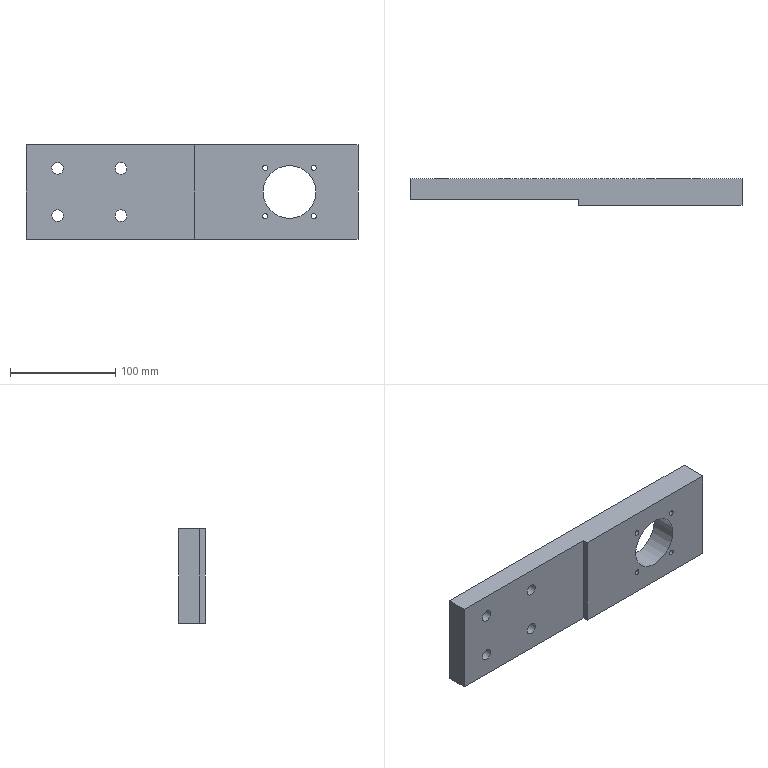Part | STEP file | SN10_003_002_PLACA | 1 solid | 17 faces | box 315 x 25 x 90 mm | volume 578161 mm3 | cylinder 9 | plane 8 | commonest cylinder face diameters 4.917 x4 11 x4 50 x1
STEP:
#1=CARTESIAN_POINT('',(0.,0.,0.));
#2=DIRECTION('',(0.,0.,1.));
#3=DIRECTION('',(1.,0.,0.));
#4=AXIS2_PLACEMENT_3D('',#1,#2,#3);
#5=CARTESIAN_POINT('',(5784.827,200.,25.137));
#6=VERTEX_POINT('',#5);
#7=CARTESIAN_POINT('',(5780.,200.,22.5));
#8=DIRECTION('',(0.,-1.,0.));
#9=DIRECTION('',(1.,0.,0.));
#10=AXIS2_PLACEMENT_3D('',#7,#8,#9);
#11=CIRCLE('',#10,5.5);
#12=CARTESIAN_POINT('',(5780.,199.9,22.5));
#13=DIRECTION('',(0.,-1.,0.));
#14=DIRECTION('',(0.8776,0.,0.4794));
#15=AXIS2_PLACEMENT_3D('',#12,#13,#14);
#16=CYLINDRICAL_SURFACE('',#15,5.5);
#17=CARTESIAN_POINT('',(-0.5,-0.1));
#18=DIRECTION('',(1.,0.));
#19=VECTOR('',#18,1.);
#20=LINE('',#17,#19);
#21=(GEOMETRIC_REPRESENTATION_CONTEXT(2)PARAMETRIC_REPRESENTATION_CONTEXT()REPRESENTATION_CONTEXT('',''));
#22=DEFINITIONAL_REPRESENTATION('',(#20),#21);
#23=PCURVE('',#16,#22);
#24=CARTESIAN_POINT('',(6065.,200.,45.));
#25=DIRECTION('',(0.,-1.,0.));
#26=DIRECTION('',(0.,0.,-1.));
#27=AXIS2_PLACEMENT_3D('',#24,#25,#26);
#28=PLANE('',#27);
#29=CARTESIAN_POINT('',(22.5,-285.));
#30=DIRECTION('',(0.,1.));
#31=AXIS2_PLACEMENT_2D('',#29,#30);
#32=CIRCLE('',#31,5.5);
#33=(GEOMETRIC_REPRESENTATION_CONTEXT(2)PARAMETRIC_REPRESENTATION_CONTEXT()REPRESENTATION_CONTEXT('',''));
#34=DEFINITIONAL_REPRESENTATION('',(#32),#33);
#35=PCURVE('',#28,#34);
#36=SURFACE_CURVE('',#11,(#23,#35),.PCURVE_S1.);
#37=EDGE_CURVE('',#6,#6,#36,.T.);
#38=ORIENTED_EDGE('',*,*,#37,.T.);
#39=CARTESIAN_POINT('',(5784.827,180.,25.137));
#40=VERTEX_POINT('',#39);
#41=CARTESIAN_POINT('',(5784.827,200.,25.137));
#42=CARTESIAN_POINT('',(5784.827,180.,25.137));
#43=B_SPLINE_CURVE_WITH_KNOTS('',1,(#41,#42),.UNSPECIFIED.,.F.,.F.,(2,2),(-0.1,19.9),.PIECEWISE_BEZIER_KNOTS.);
#44=CARTESIAN_POINT('',(6.283,0.));
#45=DIRECTION('',(0.,1.));
#46=VECTOR('',#45,1.);
#47=LINE('',#44,#46);
#48=(GEOMETRIC_REPRESENTATION_CONTEXT(2)PARAMETRIC_REPRESENTATION_CONTEXT()REPRESENTATION_CONTEXT('',''));
#49=DEFINITIONAL_REPRESENTATION('',(#47),#48);
#50=PCURVE('',#16,#49);
#51=CARTESIAN_POINT('',(0.,0.));
#52=DIRECTION('',(0.,1.));
#53=VECTOR('',#52,1.);
#54=LINE('',#51,#53);
#55=(GEOMETRIC_REPRESENTATION_CONTEXT(2)PARAMETRIC_REPRESENTATION_CONTEXT()REPRESENTATION_CONTEXT('',''));
#56=DEFINITIONAL_REPRESENTATION('',(#54),#55);
#57=PCURVE('',#16,#56);
#58=SEAM_CURVE('',#43,(#50,#57),.PCURVE_S1.);
#59=EDGE_CURVE('',#6,#40,#58,.T.);
#60=ORIENTED_EDGE('',*,*,#59,.T.);
#61=CARTESIAN_POINT('',(5780.,180.,22.5));
#62=DIRECTION('',(0.,-1.,0.));
#63=DIRECTION('',(1.,0.,0.));
#64=AXIS2_PLACEMENT_3D('',#61,#62,#63);
#65=CIRCLE('',#64,5.5);
#66=CARTESIAN_POINT('',(-0.5,19.9));
#67=DIRECTION('',(1.,0.));
#68=VECTOR('',#67,1.);
#69=LINE('',#66,#68);
#70=(GEOMETRIC_REPRESENTATION_CONTEXT(2)PARAMETRIC_REPRESENTATION_CONTEXT()REPRESENTATION_CONTEXT('',''));
#71=DEFINITIONAL_REPRESENTATION('',(#69),#70);
#72=PCURVE('',#16,#71);
#73=CARTESIAN_POINT('',(5750.,180.,45.));
#74=DIRECTION('',(0.,1.,0.));
#75=DIRECTION('',(0.,0.,1.));
#76=AXIS2_PLACEMENT_3D('',#73,#74,#75);
#77=PLANE('',#76);
#78=CARTESIAN_POINT('',(-22.5,35.5));
#79=CARTESIAN_POINT('',(-12.974,35.5));
#80=CARTESIAN_POINT('',(-17.737,27.25));
#81=CARTESIAN_POINT('',(-22.5,19.));
#82=CARTESIAN_POINT('',(-27.263,27.25));
#83=CARTESIAN_POINT('',(-32.026,35.5));
#84=CARTESIAN_POINT('',(-22.5,35.5));
#85=(BOUNDED_CURVE()B_SPLINE_CURVE(2,(#78,#79,#80,#81,#82,#83,#84),.UNSPECIFIED.,.T.,.F.)B_SPLINE_CURVE_WITH_KNOTS((1,2,2,2,2,1),(-2.094,0.,2.094,4.189,6.283,8.378),.UNSPECIFIED.)CURVE()GEOMETRIC_REPRESENTATION_ITEM()RATIONAL_B_SPLINE_CURVE((1.,0.5,1.,0.5,1.,0.5,1.))REPRESENTATION_ITEM(''));
#86=(GEOMETRIC_REPRESENTATION_CONTEXT(2)PARAMETRIC_REPRESENTATION_CONTEXT()REPRESENTATION_CONTEXT('',''));
#87=DEFINITIONAL_REPRESENTATION('',(#85),#86);
#88=PCURVE('',#77,#87);
#89=SURFACE_CURVE('',#65,(#72,#88),.PCURVE_S1.);
#90=EDGE_CURVE('',#40,#40,#89,.T.);
#91=ORIENTED_EDGE('',*,*,#90,.F.);
#92=ORIENTED_EDGE('',*,*,#59,.F.);
#93=EDGE_LOOP('',(#38,#60,#91,#92));
#94=FACE_BOUND('',#93,.F.);
#95=ADVANCED_FACE('',(#94),#16,.F.);
#96=CARTESIAN_POINT('',(6065.,175.,-45.));
#97=VERTEX_POINT('',#96);
#98=CARTESIAN_POINT('',(6065.,200.,-45.));
#99=VERTEX_POINT('',#98);
#100=CARTESIAN_POINT('',(6065.,175.,-45.));
#101=DIRECTION('',(0.,1.,0.));
#102=VECTOR('',#101,1.);
#103=LINE('',#100,#102);
#104=CARTESIAN_POINT('',(6065.,175.,45.));
#105=DIRECTION('',(-1.,0.,0.));
#106=DIRECTION('',(0.,0.,1.));
#107=AXIS2_PLACEMENT_3D('',#104,#105,#106);
#108=PLANE('',#107);
#109=CARTESIAN_POINT('',(-90.,0.));
#110=DIRECTION('',(0.,1.));
#111=VECTOR('',#110,1.);
#112=LINE('',#109,#111);
#113=(GEOMETRIC_REPRESENTATION_CONTEXT(2)PARAMETRIC_REPRESENTATION_CONTEXT()REPRESENTATION_CONTEXT('',''));
#114=DEFINITIONAL_REPRESENTATION('',(#112),#113);
#115=PCURVE('',#108,#114);
#116=CARTESIAN_POINT('',(0.,0.,-45.));
#117=DIRECTION('',(0.,0.,1.));
#118=DIRECTION('',(1.,0.,0.));
#119=AXIS2_PLACEMENT_3D('',#116,#117,#118);
#120=PLANE('',#119);
#121=CARTESIAN_POINT('',(6065.,175.));
#122=DIRECTION('',(0.,1.));
#123=VECTOR('',#122,1.);
#124=LINE('',#121,#123);
#125=(GEOMETRIC_REPRESENTATION_CONTEXT(2)PARAMETRIC_REPRESENTATION_CONTEXT()REPRESENTATION_CONTEXT('',''));
#126=DEFINITIONAL_REPRESENTATION('',(#124),#125);
#127=PCURVE('',#120,#126);
#128=SURFACE_CURVE('',#103,(#115,#127),.PCURVE_S1.);
#129=EDGE_CURVE('',#97,#99,#128,.T.);
#130=ORIENTED_EDGE('',*,*,#129,.T.);
#131=CARTESIAN_POINT('',(6065.,200.,45.));
#132=VERTEX_POINT('',#131);
#133=CARTESIAN_POINT('',(6065.,200.,45.));
#134=DIRECTION('',(0.,0.,-1.));
#135=VECTOR('',#134,1.);
#136=LINE('',#133,#135);
#137=CARTESIAN_POINT('',(0.,25.));
#138=DIRECTION('',(-1.,0.));
#139=VECTOR('',#138,1.);
#140=LINE('',#137,#139);
#141=(GEOMETRIC_REPRESENTATION_CONTEXT(2)PARAMETRIC_REPRESENTATION_CONTEXT()REPRESENTATION_CONTEXT('',''));
#142=DEFINITIONAL_REPRESENTATION('',(#140),#141);
#143=PCURVE('',#108,#142);
#144=CARTESIAN_POINT('',(0.,0.));
#145=DIRECTION('',(1.,0.));
#146=VECTOR('',#145,1.);
#147=LINE('',#144,#146);
#148=(GEOMETRIC_REPRESENTATION_CONTEXT(2)PARAMETRIC_REPRESENTATION_CONTEXT()REPRESENTATION_CONTEXT('',''));
#149=DEFINITIONAL_REPRESENTATION('',(#147),#148);
#150=PCURVE('',#28,#149);
#151=SURFACE_CURVE('',#136,(#143,#150),.PCURVE_S1.);
#152=EDGE_CURVE('',#132,#99,#151,.T.);
#153=ORIENTED_EDGE('',*,*,#152,.F.);
#154=CARTESIAN_POINT('',(6065.,175.,45.));
#155=VERTEX_POINT('',#154);
#156=CARTESIAN_POINT('',(6065.,175.,45.));
#157=DIRECTION('',(0.,1.,0.));
#158=VECTOR('',#157,1.);
#159=LINE('',#156,#158);
#160=CARTESIAN_POINT('',(0.,0.));
#161=DIRECTION('',(0.,1.));
#162=VECTOR('',#161,1.);
#163=LINE('',#160,#162);
#164=(GEOMETRIC_REPRESENTATION_CONTEXT(2)PARAMETRIC_REPRESENTATION_CONTEXT()REPRESENTATION_CONTEXT('',''));
#165=DEFINITIONAL_REPRESENTATION('',(#163),#164);
#166=PCURVE('',#108,#165);
#167=CARTESIAN_POINT('',(0.,0.,45.));
#168=DIRECTION('',(0.,0.,1.));
#169=DIRECTION('',(1.,0.,0.));
#170=AXIS2_PLACEMENT_3D('',#167,#168,#169);
#171=PLANE('',#170);
#172=CARTESIAN_POINT('',(6065.,175.));
#173=DIRECTION('',(0.,1.));
#174=VECTOR('',#173,1.);
#175=LINE('',#172,#174);
#176=(GEOMETRIC_REPRESENTATION_CONTEXT(2)PARAMETRIC_REPRESENTATION_CONTEXT()REPRESENTATION_CONTEXT('',''));
#177=DEFINITIONAL_REPRESENTATION('',(#175),#176);
#178=PCURVE('',#171,#177);
#179=SURFACE_CURVE('',#159,(#166,#178),.PCURVE_S1.);
#180=EDGE_CURVE('',#155,#132,#179,.T.);
#181=ORIENTED_EDGE('',*,*,#180,.F.);
#182=CARTESIAN_POINT('',(6065.,175.,45.));
#183=DIRECTION('',(0.,0.,-1.));
#184=VECTOR('',#183,1.);
#185=LINE('',#182,#184);
#186=CARTESIAN_POINT('',(0.,0.));
#187=DIRECTION('',(-1.,0.));
#188=VECTOR('',#187,1.);
#189=LINE('',#186,#188);
#190=(GEOMETRIC_REPRESENTATION_CONTEXT(2)PARAMETRIC_REPRESENTATION_CONTEXT()REPRESENTATION_CONTEXT('',''));
#191=DEFINITIONAL_REPRESENTATION('',(#189),#190);
#192=PCURVE('',#108,#191);
#193=CARTESIAN_POINT('',(5910.,175.,45.));
#194=DIRECTION('',(0.,1.,0.));
#195=DIRECTION('',(0.,0.,1.));
#196=AXIS2_PLACEMENT_3D('',#193,#194,#195);
#197=PLANE('',#196);
#198=CARTESIAN_POINT('',(0.,155.));
#199=DIRECTION('',(-1.,0.));
#200=VECTOR('',#199,1.);
#201=LINE('',#198,#200);
#202=(GEOMETRIC_REPRESENTATION_CONTEXT(2)PARAMETRIC_REPRESENTATION_CONTEXT()REPRESENTATION_CONTEXT('',''));
#203=DEFINITIONAL_REPRESENTATION('',(#201),#202);
#204=PCURVE('',#197,#203);
#205=SURFACE_CURVE('',#185,(#192,#204),.PCURVE_S1.);
#206=EDGE_CURVE('',#155,#97,#205,.T.);
#207=ORIENTED_EDGE('',*,*,#206,.T.);
#208=EDGE_LOOP('',(#130,#153,#181,#207));
#209=FACE_BOUND('',#208,.T.);
#210=ADVANCED_FACE('',(#209),#108,.F.);
#211=CARTESIAN_POINT('',(5750.,200.,-45.));
#212=VERTEX_POINT('',#211);
#213=CARTESIAN_POINT('',(5750.,180.,-45.));
#214=VERTEX_POINT('',#213);
#215=CARTESIAN_POINT('',(5750.,200.,-45.));
#216=DIRECTION('',(0.,-1.,0.));
#217=VECTOR('',#216,1.);
#218=LINE('',#215,#217);
#219=CARTESIAN_POINT('',(5750.,200.));
#220=DIRECTION('',(0.,-1.));
#221=VECTOR('',#220,1.);
#222=LINE('',#219,#221);
#223=(GEOMETRIC_REPRESENTATION_CONTEXT(2)PARAMETRIC_REPRESENTATION_CONTEXT()REPRESENTATION_CONTEXT('',''));
#224=DEFINITIONAL_REPRESENTATION('',(#222),#223);
#225=PCURVE('',#120,#224);
#226=CARTESIAN_POINT('',(5750.,200.,45.));
#227=DIRECTION('',(1.,0.,0.));
#228=DIRECTION('',(0.,0.,-1.));
#229=AXIS2_PLACEMENT_3D('',#226,#227,#228);
#230=PLANE('',#229);
#231=CARTESIAN_POINT('',(90.,0.));
#232=DIRECTION('',(0.,-1.));
#233=VECTOR('',#232,1.);
#234=LINE('',#231,#233);
#235=(GEOMETRIC_REPRESENTATION_CONTEXT(2)PARAMETRIC_REPRESENTATION_CONTEXT()REPRESENTATION_CONTEXT('',''));
#236=DEFINITIONAL_REPRESENTATION('',(#234),#235);
#237=PCURVE('',#230,#236);
#238=SURFACE_CURVE('',#218,(#225,#237),.PCURVE_S1.);
#239=EDGE_CURVE('',#212,#214,#238,.T.);
#240=ORIENTED_EDGE('',*,*,#239,.F.);
#241=CARTESIAN_POINT('',(6065.,200.,-45.));
#242=DIRECTION('',(-1.,0.,0.));
#243=VECTOR('',#242,1.);
#244=LINE('',#241,#243);
#245=CARTESIAN_POINT('',(6065.,200.));
#246=DIRECTION('',(-1.,0.));
#247=VECTOR('',#246,1.);
#248=LINE('',#245,#247);
#249=(GEOMETRIC_REPRESENTATION_CONTEXT(2)PARAMETRIC_REPRESENTATION_CONTEXT()REPRESENTATION_CONTEXT('',''));
#250=DEFINITIONAL_REPRESENTATION('',(#248),#249);
#251=PCURVE('',#120,#250);
#252=CARTESIAN_POINT('',(90.,0.));
#253=DIRECTION('',(0.,-1.));
#254=VECTOR('',#253,1.);
#255=LINE('',#252,#254);
#256=(GEOMETRIC_REPRESENTATION_CONTEXT(2)PARAMETRIC_REPRESENTATION_CONTEXT()REPRESENTATION_CONTEXT('',''));
#257=DEFINITIONAL_REPRESENTATION('',(#255),#256);
#258=PCURVE('',#28,#257);
#259=SURFACE_CURVE('',#244,(#251,#258),.PCURVE_S1.);
#260=EDGE_CURVE('',#99,#212,#259,.T.);
#261=ORIENTED_EDGE('',*,*,#260,.F.);
#262=ORIENTED_EDGE('',*,*,#129,.F.);
#263=CARTESIAN_POINT('',(5910.,175.,-45.));
#264=VERTEX_POINT('',#263);
#265=CARTESIAN_POINT('',(5910.,175.,-45.));
#266=DIRECTION('',(1.,0.,0.));
#267=VECTOR('',#266,1.);
#268=LINE('',#265,#267);
#269=CARTESIAN_POINT('',(5910.,175.));
#270=DIRECTION('',(1.,0.));
#271=VECTOR('',#270,1.);
#272=LINE('',#269,#271);
#273=(GEOMETRIC_REPRESENTATION_CONTEXT(2)PARAMETRIC_REPRESENTATION_CONTEXT()REPRESENTATION_CONTEXT('',''));
#274=DEFINITIONAL_REPRESENTATION('',(#272),#273);
#275=PCURVE('',#120,#274);
#276=CARTESIAN_POINT('',(-90.,0.));
#277=DIRECTION('',(0.,1.));
#278=VECTOR('',#277,1.);
#279=LINE('',#276,#278);
#280=(GEOMETRIC_REPRESENTATION_CONTEXT(2)PARAMETRIC_REPRESENTATION_CONTEXT()REPRESENTATION_CONTEXT('',''));
#281=DEFINITIONAL_REPRESENTATION('',(#279),#280);
#282=PCURVE('',#197,#281);
#283=SURFACE_CURVE('',#268,(#275,#282),.PCURVE_S1.);
#284=EDGE_CURVE('',#264,#97,#283,.T.);
#285=ORIENTED_EDGE('',*,*,#284,.F.);
#286=CARTESIAN_POINT('',(5910.,180.,-45.));
#287=VERTEX_POINT('',#286);
#288=CARTESIAN_POINT('',(5910.,180.,-45.));
#289=DIRECTION('',(0.,-1.,0.));
#290=VECTOR('',#289,1.);
#291=LINE('',#288,#290);
#292=CARTESIAN_POINT('',(5910.,180.));
#293=DIRECTION('',(0.,-1.));
#294=VECTOR('',#293,1.);
#295=LINE('',#292,#294);
#296=(GEOMETRIC_REPRESENTATION_CONTEXT(2)PARAMETRIC_REPRESENTATION_CONTEXT()REPRESENTATION_CONTEXT('',''));
#297=DEFINITIONAL_REPRESENTATION('',(#295),#296);
#298=PCURVE('',#120,#297);
#299=CARTESIAN_POINT('',(5910.,180.,45.));
#300=DIRECTION('',(1.,0.,0.));
#301=DIRECTION('',(0.,0.,-1.));
#302=AXIS2_PLACEMENT_3D('',#299,#300,#301);
#303=PLANE('',#302);
#304=CARTESIAN_POINT('',(90.,0.));
#305=DIRECTION('',(0.,-1.));
#306=VECTOR('',#305,1.);
#307=LINE('',#304,#306);
#308=(GEOMETRIC_REPRESENTATION_CONTEXT(2)PARAMETRIC_REPRESENTATION_CONTEXT()REPRESENTATION_CONTEXT('',''));
#309=DEFINITIONAL_REPRESENTATION('',(#307),#308);
#310=PCURVE('',#303,#309);
#311=SURFACE_CURVE('',#291,(#298,#310),.PCURVE_S1.);
#312=EDGE_CURVE('',#287,#264,#311,.T.);
#313=ORIENTED_EDGE('',*,*,#312,.F.);
#314=CARTESIAN_POINT('',(5750.,180.,-45.));
#315=DIRECTION('',(1.,0.,0.));
#316=VECTOR('',#315,1.);
#317=LINE('',#314,#316);
#318=CARTESIAN_POINT('',(5750.,180.));
#319=DIRECTION('',(1.,0.));
#320=VECTOR('',#319,1.);
#321=LINE('',#318,#320);
#322=(GEOMETRIC_REPRESENTATION_CONTEXT(2)PARAMETRIC_REPRESENTATION_CONTEXT()REPRESENTATION_CONTEXT('',''));
#323=DEFINITIONAL_REPRESENTATION('',(#321),#322);
#324=PCURVE('',#120,#323);
#325=CARTESIAN_POINT('',(-90.,0.));
#326=DIRECTION('',(0.,1.));
#327=VECTOR('',#326,1.);
#328=LINE('',#325,#327);
#329=(GEOMETRIC_REPRESENTATION_CONTEXT(2)PARAMETRIC_REPRESENTATION_CONTEXT()REPRESENTATION_CONTEXT('',''));
#330=DEFINITIONAL_REPRESENTATION('',(#328),#329);
#331=PCURVE('',#77,#330);
#332=SURFACE_CURVE('',#317,(#324,#331),.PCURVE_S1.);
#333=EDGE_CURVE('',#214,#287,#332,.T.);
#334=ORIENTED_EDGE('',*,*,#333,.F.);
#335=EDGE_LOOP('',(#240,#261,#262,#285,#313,#334));
#336=FACE_BOUND('',#335,.T.);
#337=ADVANCED_FACE('',(#336),#120,.F.);
#338=CARTESIAN_POINT('',(6020.823,200.,21.802));
#339=VERTEX_POINT('',#338);
#340=CARTESIAN_POINT('',(6022.981,200.,22.981));
#341=DIRECTION('',(0.,-1.,0.));
#342=DIRECTION('',(1.,0.,0.));
#343=AXIS2_PLACEMENT_3D('',#340,#341,#342);
#344=CIRCLE('',#343,2.458);
#345=CARTESIAN_POINT('',(6022.981,199.9,22.981));
#346=DIRECTION('',(0.,-1.,0.));
#347=DIRECTION('',(0.8776,0.,0.4794));
#348=AXIS2_PLACEMENT_3D('',#345,#346,#347);
#349=CYLINDRICAL_SURFACE('',#348,2.458);
#350=CARTESIAN_POINT('',(-0.5,-0.1));
#351=DIRECTION('',(1.,0.));
#352=VECTOR('',#351,1.);
#353=LINE('',#350,#352);
#354=(GEOMETRIC_REPRESENTATION_CONTEXT(2)PARAMETRIC_REPRESENTATION_CONTEXT()REPRESENTATION_CONTEXT('',''));
#355=DEFINITIONAL_REPRESENTATION('',(#353),#354);
#356=PCURVE('',#349,#355);
#357=CARTESIAN_POINT('',(22.019,-42.019));
#358=DIRECTION('',(0.,1.));
#359=AXIS2_PLACEMENT_2D('',#357,#358);
#360=CIRCLE('',#359,2.458);
#361=(GEOMETRIC_REPRESENTATION_CONTEXT(2)PARAMETRIC_REPRESENTATION_CONTEXT()REPRESENTATION_CONTEXT('',''));
#362=DEFINITIONAL_REPRESENTATION('',(#360),#361);
#363=PCURVE('',#28,#362);
#364=SURFACE_CURVE('',#344,(#356,#363),.PCURVE_S1.);
#365=EDGE_CURVE('',#339,#339,#364,.T.);
#366=ORIENTED_EDGE('',*,*,#365,.T.);
#367=CARTESIAN_POINT('',(6020.823,175.,21.802));
#368=VERTEX_POINT('',#367);
#369=CARTESIAN_POINT('',(6020.823,200.,21.802));
#370=CARTESIAN_POINT('',(6020.823,175.,21.802));
#371=B_SPLINE_CURVE_WITH_KNOTS('',1,(#369,#370),.UNSPECIFIED.,.F.,.F.,(2,2),(-0.1,24.9),.PIECEWISE_BEZIER_KNOTS.);
#372=CARTESIAN_POINT('',(9.425,0.));
#373=DIRECTION('',(0.,1.));
#374=VECTOR('',#373,1.);
#375=LINE('',#372,#374);
#376=(GEOMETRIC_REPRESENTATION_CONTEXT(2)PARAMETRIC_REPRESENTATION_CONTEXT()REPRESENTATION_CONTEXT('',''));
#377=DEFINITIONAL_REPRESENTATION('',(#375),#376);
#378=PCURVE('',#349,#377);
#379=CARTESIAN_POINT('',(3.142,0.));
#380=DIRECTION('',(0.,1.));
#381=VECTOR('',#380,1.);
#382=LINE('',#379,#381);
#383=(GEOMETRIC_REPRESENTATION_CONTEXT(2)PARAMETRIC_REPRESENTATION_CONTEXT()REPRESENTATION_CONTEXT('',''));
#384=DEFINITIONAL_REPRESENTATION('',(#382),#383);
#385=PCURVE('',#349,#384);
#386=SEAM_CURVE('',#371,(#378,#385),.PCURVE_S1.);
#387=EDGE_CURVE('',#339,#368,#386,.T.);
#388=ORIENTED_EDGE('',*,*,#387,.T.);
#389=CARTESIAN_POINT('',(6022.981,175.,22.981));
#390=DIRECTION('',(0.,-1.,0.));
#391=DIRECTION('',(1.,0.,0.));
#392=AXIS2_PLACEMENT_3D('',#389,#390,#391);
#393=CIRCLE('',#392,2.458);
#394=CARTESIAN_POINT('',(-0.5,24.9));
#395=DIRECTION('',(1.,0.));
#396=VECTOR('',#395,1.);
#397=LINE('',#394,#396);
#398=(GEOMETRIC_REPRESENTATION_CONTEXT(2)PARAMETRIC_REPRESENTATION_CONTEXT()REPRESENTATION_CONTEXT('',''));
#399=DEFINITIONAL_REPRESENTATION('',(#397),#398);
#400=PCURVE('',#349,#399);
#401=CARTESIAN_POINT('',(-22.019,115.439));
#402=CARTESIAN_POINT('',(-17.761,115.439));
#403=CARTESIAN_POINT('',(-19.89,111.752));
#404=CARTESIAN_POINT('',(-22.019,108.064));
#405=CARTESIAN_POINT('',(-24.148,111.752));
#406=CARTESIAN_POINT('',(-26.277,115.439));
#407=CARTESIAN_POINT('',(-22.019,115.439));
#408=(BOUNDED_CURVE()B_SPLINE_CURVE(2,(#401,#402,#403,#404,#405,#406,#407),.UNSPECIFIED.,.T.,.F.)B_SPLINE_CURVE_WITH_KNOTS((1,2,2,2,2,1),(-2.094,0.,2.094,4.189,6.283,8.378),.UNSPECIFIED.)CURVE()GEOMETRIC_REPRESENTATION_ITEM()RATIONAL_B_SPLINE_CURVE((1.,0.5,1.,0.5,1.,0.5,1.))REPRESENTATION_ITEM(''));
#409=(GEOMETRIC_REPRESENTATION_CONTEXT(2)PARAMETRIC_REPRESENTATION_CONTEXT()REPRESENTATION_CONTEXT('',''));
#410=DEFINITIONAL_REPRESENTATION('',(#408),#409);
#411=PCURVE('',#197,#410);
#412=SURFACE_CURVE('',#393,(#400,#411),.PCURVE_S1.);
#413=EDGE_CURVE('',#368,#368,#412,.T.);
#414=ORIENTED_EDGE('',*,*,#413,.F.);
#415=ORIENTED_EDGE('',*,*,#387,.F.);
#416=EDGE_LOOP('',(#366,#388,#414,#415));
#417=FACE_BOUND('',#416,.F.);
#418=ADVANCED_FACE('',(#417),#349,.F.);
#419=CARTESIAN_POINT('',(5975.,200.,0.));
#420=VERTEX_POINT('',#419);
#421=CARTESIAN_POINT('',(6000.,200.,0.));
#422=DIRECTION('',(0.,-1.,0.));
#423=DIRECTION('',(1.,0.,0.));
#424=AXIS2_PLACEMENT_3D('',#421,#422,#423);
#425=CIRCLE('',#424,25.);
#426=CARTESIAN_POINT('',(6000.,188.16,0.));
#427=DIRECTION('',(0.,-1.,0.));
#428=DIRECTION('',(1.,0.,0.));
#429=AXIS2_PLACEMENT_3D('',#426,#427,#428);
#430=CYLINDRICAL_SURFACE('',#429,25.);
#431=CARTESIAN_POINT('',(0.,-11.84));
#432=DIRECTION('',(1.,0.));
#433=VECTOR('',#432,1.);
#434=LINE('',#431,#433);
#435=(GEOMETRIC_REPRESENTATION_CONTEXT(2)PARAMETRIC_REPRESENTATION_CONTEXT()REPRESENTATION_CONTEXT('',''));
#436=DEFINITIONAL_REPRESENTATION('',(#434),#435);
#437=PCURVE('',#430,#436);
#438=CARTESIAN_POINT('',(45.,-65.));
#439=DIRECTION('',(0.,1.));
#440=AXIS2_PLACEMENT_2D('',#438,#439);
#441=CIRCLE('',#440,25.);
#442=(GEOMETRIC_REPRESENTATION_CONTEXT(2)PARAMETRIC_REPRESENTATION_CONTEXT()REPRESENTATION_CONTEXT('',''));
#443=DEFINITIONAL_REPRESENTATION('',(#441),#442);
#444=PCURVE('',#28,#443);
#445=SURFACE_CURVE('',#425,(#437,#444),.PCURVE_S1.);
#446=EDGE_CURVE('',#420,#420,#445,.T.);
#447=ORIENTED_EDGE('',*,*,#446,.T.);
#448=CARTESIAN_POINT('',(5975.,175.,0.));
#449=VERTEX_POINT('',#448);
#450=CARTESIAN_POINT('',(5975.,200.,0.));
#451=CARTESIAN_POINT('',(5975.,175.,0.));
#452=B_SPLINE_CURVE_WITH_KNOTS('',1,(#450,#451),.UNSPECIFIED.,.F.,.F.,(2,2),(-11.84,13.16),.PIECEWISE_BEZIER_KNOTS.);
#453=CARTESIAN_POINT('',(9.425,0.));
#454=DIRECTION('',(0.,1.));
#455=VECTOR('',#454,1.);
#456=LINE('',#453,#455);
#457=(GEOMETRIC_REPRESENTATION_CONTEXT(2)PARAMETRIC_REPRESENTATION_CONTEXT()REPRESENTATION_CONTEXT('',''));
#458=DEFINITIONAL_REPRESENTATION('',(#456),#457);
#459=PCURVE('',#430,#458);
#460=CARTESIAN_POINT('',(3.142,0.));
#461=DIRECTION('',(0.,1.));
#462=VECTOR('',#461,1.);
#463=LINE('',#460,#462);
#464=(GEOMETRIC_REPRESENTATION_CONTEXT(2)PARAMETRIC_REPRESENTATION_CONTEXT()REPRESENTATION_CONTEXT('',''));
#465=DEFINITIONAL_REPRESENTATION('',(#463),#464);
#466=PCURVE('',#430,#465);
#467=SEAM_CURVE('',#452,(#459,#466),.PCURVE_S1.);
#468=EDGE_CURVE('',#420,#449,#467,.T.);
#469=ORIENTED_EDGE('',*,*,#468,.T.);
#470=CARTESIAN_POINT('',(6000.,175.,0.));
#471=DIRECTION('',(0.,-1.,0.));
#472=DIRECTION('',(1.,0.,0.));
#473=AXIS2_PLACEMENT_3D('',#470,#471,#472);
#474=CIRCLE('',#473,25.);
#475=CARTESIAN_POINT('',(0.,13.16));
#476=DIRECTION('',(1.,0.));
#477=VECTOR('',#476,1.);
#478=LINE('',#475,#477);
#479=(GEOMETRIC_REPRESENTATION_CONTEXT(2)PARAMETRIC_REPRESENTATION_CONTEXT()REPRESENTATION_CONTEXT('',''));
#480=DEFINITIONAL_REPRESENTATION('',(#478),#479);
#481=PCURVE('',#430,#480);
#482=CARTESIAN_POINT('',(-45.,115.));
#483=CARTESIAN_POINT('',(-1.699,115.));
#484=CARTESIAN_POINT('',(-23.349,77.5));
#485=CARTESIAN_POINT('',(-45.,40.));
#486=CARTESIAN_POINT('',(-66.651,77.5));
#487=CARTESIAN_POINT('',(-88.301,115.));
#488=CARTESIAN_POINT('',(-45.,115.));
#489=(BOUNDED_CURVE()B_SPLINE_CURVE(2,(#482,#483,#484,#485,#486,#487,#488),.UNSPECIFIED.,.T.,.F.)B_SPLINE_CURVE_WITH_KNOTS((1,2,2,2,2,1),(-2.094,0.,2.094,4.189,6.283,8.378),.UNSPECIFIED.)CURVE()GEOMETRIC_REPRESENTATION_ITEM()RATIONAL_B_SPLINE_CURVE((1.,0.5,1.,0.5,1.,0.5,1.))REPRESENTATION_ITEM(''));
#490=(GEOMETRIC_REPRESENTATION_CONTEXT(2)PARAMETRIC_REPRESENTATION_CONTEXT()REPRESENTATION_CONTEXT('',''));
#491=DEFINITIONAL_REPRESENTATION('',(#489),#490);
#492=PCURVE('',#197,#491);
#493=SURFACE_CURVE('',#474,(#481,#492),.PCURVE_S1.);
#494=EDGE_CURVE('',#449,#449,#493,.T.);
#495=ORIENTED_EDGE('',*,*,#494,.F.);
#496=ORIENTED_EDGE('',*,*,#468,.F.);
#497=EDGE_LOOP('',(#447,#469,#495,#496));
#498=FACE_BOUND('',#497,.F.);
#499=ADVANCED_FACE('',(#498),#430,.F.);
#500=CARTESIAN_POINT('',(6024.16,200.,-25.139));
#501=VERTEX_POINT('',#500);
#502=CARTESIAN_POINT('',(6022.981,200.,-22.981));
#503=DIRECTION('',(0.,-1.,0.));
#504=DIRECTION('',(1.,0.,0.));
#505=AXIS2_PLACEMENT_3D('',#502,#503,#504);
#506=CIRCLE('',#505,2.458);
#507=CARTESIAN_POINT('',(6022.981,199.9,-22.981));
#508=DIRECTION('',(0.,-1.,0.));
#509=DIRECTION('',(0.4794,0.,-0.8776));
#510=AXIS2_PLACEMENT_3D('',#507,#508,#509);
#511=CYLINDRICAL_SURFACE('',#510,2.458);
#512=CARTESIAN_POINT('',(1.071,-0.1));
#513=DIRECTION('',(1.,0.));
#514=VECTOR('',#513,1.);
#515=LINE('',#512,#514);
#516=(GEOMETRIC_REPRESENTATION_CONTEXT(2)PARAMETRIC_REPRESENTATION_CONTEXT()REPRESENTATION_CONTEXT('',''));
#517=DEFINITIONAL_REPRESENTATION('',(#515),#516);
#518=PCURVE('',#511,#517);
#519=CARTESIAN_POINT('',(67.981,-42.019));
#520=DIRECTION('',(0.,1.));
#521=AXIS2_PLACEMENT_2D('',#519,#520);
#522=CIRCLE('',#521,2.458);
#523=(GEOMETRIC_REPRESENTATION_CONTEXT(2)PARAMETRIC_REPRESENTATION_CONTEXT()REPRESENTATION_CONTEXT('',''));
#524=DEFINITIONAL_REPRESENTATION('',(#522),#523);
#525=PCURVE('',#28,#524);
#526=SURFACE_CURVE('',#506,(#518,#525),.PCURVE_S1.);
#527=EDGE_CURVE('',#501,#501,#526,.T.);
#528=ORIENTED_EDGE('',*,*,#527,.T.);
#529=CARTESIAN_POINT('',(6024.16,175.,-25.139));
#530=VERTEX_POINT('',#529);
#531=CARTESIAN_POINT('',(6024.16,200.,-25.139));
#532=CARTESIAN_POINT('',(6024.16,175.,-25.139));
#533=B_SPLINE_CURVE_WITH_KNOTS('',1,(#531,#532),.UNSPECIFIED.,.F.,.F.,(2,2),(-0.1,24.9),.PIECEWISE_BEZIER_KNOTS.);
#534=CARTESIAN_POINT('',(12.566,0.));
#535=DIRECTION('',(0.,1.));
#536=VECTOR('',#535,1.);
#537=LINE('',#534,#536);
#538=(GEOMETRIC_REPRESENTATION_CONTEXT(2)PARAMETRIC_REPRESENTATION_CONTEXT()REPRESENTATION_CONTEXT('',''));
#539=DEFINITIONAL_REPRESENTATION('',(#537),#538);
#540=PCURVE('',#511,#539);
#541=CARTESIAN_POINT('',(6.283,0.));
#542=DIRECTION('',(0.,1.));
#543=VECTOR('',#542,1.);
#544=LINE('',#541,#543);
#545=(GEOMETRIC_REPRESENTATION_CONTEXT(2)PARAMETRIC_REPRESENTATION_CONTEXT()REPRESENTATION_CONTEXT('',''));
#546=DEFINITIONAL_REPRESENTATION('',(#544),#545);
#547=PCURVE('',#511,#546);
#548=SEAM_CURVE('',#533,(#540,#547),.PCURVE_S1.);
#549=EDGE_CURVE('',#501,#530,#548,.T.);
#550=ORIENTED_EDGE('',*,*,#549,.T.);
#551=CARTESIAN_POINT('',(6022.981,175.,-22.981));
#552=DIRECTION('',(0.,-1.,0.));
#553=DIRECTION('',(1.,0.,0.));
#554=AXIS2_PLACEMENT_3D('',#551,#552,#553);
#555=CIRCLE('',#554,2.458);
#556=CARTESIAN_POINT('',(1.071,24.9));
#557=DIRECTION('',(1.,0.));
#558=VECTOR('',#557,1.);
#559=LINE('',#556,#558);
#560=(GEOMETRIC_REPRESENTATION_CONTEXT(2)PARAMETRIC_REPRESENTATION_CONTEXT()REPRESENTATION_CONTEXT('',''));
#561=DEFINITIONAL_REPRESENTATION('',(#559),#560);
#562=PCURVE('',#511,#561);
#563=CARTESIAN_POINT('',(-67.981,115.439));
#564=CARTESIAN_POINT('',(-63.723,115.439));
#565=CARTESIAN_POINT('',(-65.852,111.752));
#566=CARTESIAN_POINT('',(-67.981,108.064));
#567=CARTESIAN_POINT('',(-70.11,111.752));
#568=CARTESIAN_POINT('',(-72.239,115.439));
#569=CARTESIAN_POINT('',(-67.981,115.439));
#570=(BOUNDED_CURVE()B_SPLINE_CURVE(2,(#563,#564,#565,#566,#567,#568,#569),.UNSPECIFIED.,.T.,.F.)B_SPLINE_CURVE_WITH_KNOTS((1,2,2,2,2,1),(-2.094,0.,2.094,4.189,6.283,8.378),.UNSPECIFIED.)CURVE()GEOMETRIC_REPRESENTATION_ITEM()RATIONAL_B_SPLINE_CURVE((1.,0.5,1.,0.5,1.,0.5,1.))REPRESENTATION_ITEM(''));
#571=(GEOMETRIC_REPRESENTATION_CONTEXT(2)PARAMETRIC_REPRESENTATION_CONTEXT()REPRESENTATION_CONTEXT('',''));
#572=DEFINITIONAL_REPRESENTATION('',(#570),#571);
#573=PCURVE('',#197,#572);
#574=SURFACE_CURVE('',#555,(#562,#573),.PCURVE_S1.);
#575=EDGE_CURVE('',#530,#530,#574,.T.);
#576=ORIENTED_EDGE('',*,*,#575,.F.);
#577=ORIENTED_EDGE('',*,*,#549,.F.);
#578=EDGE_LOOP('',(#528,#550,#576,#577));
#579=FACE_BOUND('',#578,.F.);
#580=ADVANCED_FACE('',(#579),#511,.F.);
#581=CARTESIAN_POINT('',(5974.861,200.,-24.16));
#582=VERTEX_POINT('',#581);
#583=CARTESIAN_POINT('',(5977.019,200.,-22.981));
#584=DIRECTION('',(0.,-1.,0.));
#585=DIRECTION('',(1.,0.,0.));
#586=AXIS2_PLACEMENT_3D('',#583,#584,#585);
#587=CIRCLE('',#586,2.458);
#588=CARTESIAN_POINT('',(5977.019,199.9,-22.981));
#589=DIRECTION('',(0.,-1.,0.));
#590=DIRECTION('',(-0.8776,0.,-0.4794));
#591=AXIS2_PLACEMENT_3D('',#588,#589,#590);
#592=CYLINDRICAL_SURFACE('',#591,2.458);
#593=CARTESIAN_POINT('',(-3.642,-0.1));
#594=DIRECTION('',(1.,0.));
#595=VECTOR('',#594,1.);
#596=LINE('',#593,#595);
#597=(GEOMETRIC_REPRESENTATION_CONTEXT(2)PARAMETRIC_REPRESENTATION_CONTEXT()REPRESENTATION_CONTEXT('',''));
#598=DEFINITIONAL_REPRESENTATION('',(#596),#597);
#599=PCURVE('',#592,#598);
#600=CARTESIAN_POINT('',(67.981,-87.981));
#601=DIRECTION('',(0.,1.));
#602=AXIS2_PLACEMENT_2D('',#600,#601);
#603=CIRCLE('',#602,2.458);
#604=(GEOMETRIC_REPRESENTATION_CONTEXT(2)PARAMETRIC_REPRESENTATION_CONTEXT()REPRESENTATION_CONTEXT('',''));
#605=DEFINITIONAL_REPRESENTATION('',(#603),#604);
#606=PCURVE('',#28,#605);
#607=SURFACE_CURVE('',#587,(#599,#606),.PCURVE_S1.);
#608=EDGE_CURVE('',#582,#582,#607,.T.);
#609=ORIENTED_EDGE('',*,*,#608,.T.);
#610=CARTESIAN_POINT('',(5974.861,175.,-24.16));
#611=VERTEX_POINT('',#610);
#612=CARTESIAN_POINT('',(5974.861,200.,-24.16));
#613=CARTESIAN_POINT('',(5974.861,175.,-24.16));
#614=B_SPLINE_CURVE_WITH_KNOTS('',1,(#612,#613),.UNSPECIFIED.,.F.,.F.,(2,2),(-0.1,24.9),.PIECEWISE_BEZIER_KNOTS.);
#615=CARTESIAN_POINT('',(6.283,0.));
#616=DIRECTION('',(0.,1.));
#617=VECTOR('',#616,1.);
#618=LINE('',#615,#617);
#619=(GEOMETRIC_REPRESENTATION_CONTEXT(2)PARAMETRIC_REPRESENTATION_CONTEXT()REPRESENTATION_CONTEXT('',''));
#620=DEFINITIONAL_REPRESENTATION('',(#618),#619);
#621=PCURVE('',#592,#620);
#622=CARTESIAN_POINT('',(0.,0.));
#623=DIRECTION('',(0.,1.));
#624=VECTOR('',#623,1.);
#625=LINE('',#622,#624);
#626=(GEOMETRIC_REPRESENTATION_CONTEXT(2)PARAMETRIC_REPRESENTATION_CONTEXT()REPRESENTATION_CONTEXT('',''));
#627=DEFINITIONAL_REPRESENTATION('',(#625),#626);
#628=PCURVE('',#592,#627);
#629=SEAM_CURVE('',#614,(#621,#628),.PCURVE_S1.);
#630=EDGE_CURVE('',#582,#611,#629,.T.);
#631=ORIENTED_EDGE('',*,*,#630,.T.);
#632=CARTESIAN_POINT('',(5977.019,175.,-22.981));
#633=DIRECTION('',(0.,-1.,0.));
#634=DIRECTION('',(1.,0.,0.));
#635=AXIS2_PLACEMENT_3D('',#632,#633,#634);
#636=CIRCLE('',#635,2.458);
#637=CARTESIAN_POINT('',(-3.642,24.9));
#638=DIRECTION('',(1.,0.));
#639=VECTOR('',#638,1.);
#640=LINE('',#637,#639);
#641=(GEOMETRIC_REPRESENTATION_CONTEXT(2)PARAMETRIC_REPRESENTATION_CONTEXT()REPRESENTATION_CONTEXT('',''));
#642=DEFINITIONAL_REPRESENTATION('',(#640),#641);
#643=PCURVE('',#592,#642);
#644=CARTESIAN_POINT('',(-67.981,69.478));
#645=CARTESIAN_POINT('',(-63.723,69.478));
#646=CARTESIAN_POINT('',(-65.852,65.79));
#647=CARTESIAN_POINT('',(-67.981,62.102));
#648=CARTESIAN_POINT('',(-70.11,65.79));
#649=CARTESIAN_POINT('',(-72.239,69.478));
#650=CARTESIAN_POINT('',(-67.981,69.478));
#651=(BOUNDED_CURVE()B_SPLINE_CURVE(2,(#644,#645,#646,#647,#648,#649,#650),.UNSPECIFIED.,.T.,.F.)B_SPLINE_CURVE_WITH_KNOTS((1,2,2,2,2,1),(-2.094,0.,2.094,4.189,6.283,8.378),.UNSPECIFIED.)CURVE()GEOMETRIC_REPRESENTATION_ITEM()RATIONAL_B_SPLINE_CURVE((1.,0.5,1.,0.5,1.,0.5,1.))REPRESENTATION_ITEM(''));
#652=(GEOMETRIC_REPRESENTATION_CONTEXT(2)PARAMETRIC_REPRESENTATION_CONTEXT()REPRESENTATION_CONTEXT('',''));
#653=DEFINITIONAL_REPRESENTATION('',(#651),#652);
#654=PCURVE('',#197,#653);
#655=SURFACE_CURVE('',#636,(#643,#654),.PCURVE_S1.);
#656=EDGE_CURVE('',#611,#611,#655,.T.);
#657=ORIENTED_EDGE('',*,*,#656,.F.);
#658=ORIENTED_EDGE('',*,*,#630,.F.);
#659=EDGE_LOOP('',(#609,#631,#657,#658));
#660=FACE_BOUND('',#659,.F.);
#661=ADVANCED_FACE('',(#660),#592,.F.);
#662=CARTESIAN_POINT('',(5975.84,200.,25.139));
#663=VERTEX_POINT('',#662);
#664=CARTESIAN_POINT('',(5977.019,200.,22.981));
#665=DIRECTION('',(0.,-1.,0.));
#666=DIRECTION('',(1.,0.,0.));
#667=AXIS2_PLACEMENT_3D('',#664,#665,#666);
#668=CIRCLE('',#667,2.458);
#669=CARTESIAN_POINT('',(5977.019,199.9,22.981));
#670=DIRECTION('',(0.,-1.,0.));
#671=DIRECTION('',(-0.4794,0.,0.8776));
#672=AXIS2_PLACEMENT_3D('',#669,#670,#671);
#673=CYLINDRICAL_SURFACE('',#672,2.458);
#674=CARTESIAN_POINT('',(-2.071,-0.1));
#675=DIRECTION('',(1.,0.));
#676=VECTOR('',#675,1.);
#677=LINE('',#674,#676);
#678=(GEOMETRIC_REPRESENTATION_CONTEXT(2)PARAMETRIC_REPRESENTATION_CONTEXT()REPRESENTATION_CONTEXT('',''));
#679=DEFINITIONAL_REPRESENTATION('',(#677),#678);
#680=PCURVE('',#673,#679);
#681=CARTESIAN_POINT('',(22.019,-87.981));
#682=DIRECTION('',(0.,1.));
#683=AXIS2_PLACEMENT_2D('',#681,#682);
#684=CIRCLE('',#683,2.458);
#685=(GEOMETRIC_REPRESENTATION_CONTEXT(2)PARAMETRIC_REPRESENTATION_CONTEXT()REPRESENTATION_CONTEXT('',''));
#686=DEFINITIONAL_REPRESENTATION('',(#684),#685);
#687=PCURVE('',#28,#686);
#688=SURFACE_CURVE('',#668,(#680,#687),.PCURVE_S1.);
#689=EDGE_CURVE('',#663,#663,#688,.T.);
#690=ORIENTED_EDGE('',*,*,#689,.T.);
#691=CARTESIAN_POINT('',(5975.84,175.,25.139));
#692=VERTEX_POINT('',#691);
#693=CARTESIAN_POINT('',(5975.84,200.,25.139));
#694=CARTESIAN_POINT('',(5975.84,175.,25.139));
#695=B_SPLINE_CURVE_WITH_KNOTS('',1,(#693,#694),.UNSPECIFIED.,.F.,.F.,(2,2),(-0.1,24.9),.PIECEWISE_BEZIER_KNOTS.);
#696=CARTESIAN_POINT('',(6.283,0.));
#697=DIRECTION('',(0.,1.));
#698=VECTOR('',#697,1.);
#699=LINE('',#696,#698);
#700=(GEOMETRIC_REPRESENTATION_CONTEXT(2)PARAMETRIC_REPRESENTATION_CONTEXT()REPRESENTATION_CONTEXT('',''));
#701=DEFINITIONAL_REPRESENTATION('',(#699),#700);
#702=PCURVE('',#673,#701);
#703=CARTESIAN_POINT('',(0.,0.));
#704=DIRECTION('',(0.,1.));
#705=VECTOR('',#704,1.);
#706=LINE('',#703,#705);
#707=(GEOMETRIC_REPRESENTATION_CONTEXT(2)PARAMETRIC_REPRESENTATION_CONTEXT()REPRESENTATION_CONTEXT('',''));
#708=DEFINITIONAL_REPRESENTATION('',(#706),#707);
#709=PCURVE('',#673,#708);
#710=SEAM_CURVE('',#695,(#702,#709),.PCURVE_S1.);
#711=EDGE_CURVE('',#663,#692,#710,.T.);
#712=ORIENTED_EDGE('',*,*,#711,.T.);
#713=CARTESIAN_POINT('',(5977.019,175.,22.981));
#714=DIRECTION('',(0.,-1.,0.));
#715=DIRECTION('',(1.,0.,0.));
#716=AXIS2_PLACEMENT_3D('',#713,#714,#715);
#717=CIRCLE('',#716,2.458);
#718=CARTESIAN_POINT('',(-2.071,24.9));
#719=DIRECTION('',(1.,0.));
#720=VECTOR('',#719,1.);
#721=LINE('',#718,#720);
#722=(GEOMETRIC_REPRESENTATION_CONTEXT(2)PARAMETRIC_REPRESENTATION_CONTEXT()REPRESENTATION_CONTEXT('',''));
#723=DEFINITIONAL_REPRESENTATION('',(#721),#722);
#724=PCURVE('',#673,#723);
#725=CARTESIAN_POINT('',(-22.019,69.478));
#726=CARTESIAN_POINT('',(-17.761,69.478));
#727=CARTESIAN_POINT('',(-19.89,65.79));
#728=CARTESIAN_POINT('',(-22.019,62.102));
#729=CARTESIAN_POINT('',(-24.148,65.79));
#730=CARTESIAN_POINT('',(-26.277,69.478));
#731=CARTESIAN_POINT('',(-22.019,69.478));
#732=(BOUNDED_CURVE()B_SPLINE_CURVE(2,(#725,#726,#727,#728,#729,#730,#731),.UNSPECIFIED.,.T.,.F.)B_SPLINE_CURVE_WITH_KNOTS((1,2,2,2,2,1),(-2.094,0.,2.094,4.189,6.283,8.378),.UNSPECIFIED.)CURVE()GEOMETRIC_REPRESENTATION_ITEM()RATIONAL_B_SPLINE_CURVE((1.,0.5,1.,0.5,1.,0.5,1.))REPRESENTATION_ITEM(''));
#733=(GEOMETRIC_REPRESENTATION_CONTEXT(2)PARAMETRIC_REPRESENTATION_CONTEXT()REPRESENTATION_CONTEXT('',''));
#734=DEFINITIONAL_REPRESENTATION('',(#732),#733);
#735=PCURVE('',#197,#734);
#736=SURFACE_CURVE('',#717,(#724,#735),.PCURVE_S1.);
#737=EDGE_CURVE('',#692,#692,#736,.T.);
#738=ORIENTED_EDGE('',*,*,#737,.F.);
#739=ORIENTED_EDGE('',*,*,#711,.F.);
#740=EDGE_LOOP('',(#690,#712,#738,#739));
#741=FACE_BOUND('',#740,.F.);
#742=ADVANCED_FACE('',(#741),#673,.F.);
#743=ORIENTED_EDGE('',*,*,#284,.T.);
#744=ORIENTED_EDGE('',*,*,#206,.F.);
#745=CARTESIAN_POINT('',(5910.,175.,45.));
#746=VERTEX_POINT('',#745);
#747=CARTESIAN_POINT('',(5910.,175.,45.));
#748=DIRECTION('',(1.,0.,0.));
#749=VECTOR('',#748,1.);
#750=LINE('',#747,#749);
#751=CARTESIAN_POINT('',(0.,0.));
#752=DIRECTION('',(0.,1.));
#753=VECTOR('',#752,1.);
#754=LINE('',#751,#753);
#755=(GEOMETRIC_REPRESENTATION_CONTEXT(2)PARAMETRIC_REPRESENTATION_CONTEXT()REPRESENTATION_CONTEXT('',''));
#756=DEFINITIONAL_REPRESENTATION('',(#754),#755);
#757=PCURVE('',#197,#756);
#758=CARTESIAN_POINT('',(5910.,175.));
#759=DIRECTION('',(1.,0.));
#760=VECTOR('',#759,1.);
#761=LINE('',#758,#760);
#762=(GEOMETRIC_REPRESENTATION_CONTEXT(2)PARAMETRIC_REPRESENTATION_CONTEXT()REPRESENTATION_CONTEXT('',''));
#763=DEFINITIONAL_REPRESENTATION('',(#761),#762);
#764=PCURVE('',#171,#763);
#765=SURFACE_CURVE('',#750,(#757,#764),.PCURVE_S1.);
#766=EDGE_CURVE('',#746,#155,#765,.T.);
#767=ORIENTED_EDGE('',*,*,#766,.F.);
#768=CARTESIAN_POINT('',(5910.,175.,45.));
#769=DIRECTION('',(0.,0.,-1.));
#770=VECTOR('',#769,1.);
#771=LINE('',#768,#770);
#772=CARTESIAN_POINT('',(0.,0.));
#773=DIRECTION('',(-1.,0.));
#774=VECTOR('',#773,1.);
#775=LINE('',#772,#774);
#776=(GEOMETRIC_REPRESENTATION_CONTEXT(2)PARAMETRIC_REPRESENTATION_CONTEXT()REPRESENTATION_CONTEXT('',''));
#777=DEFINITIONAL_REPRESENTATION('',(#775),#776);
#778=PCURVE('',#197,#777);
#779=CARTESIAN_POINT('',(0.,-5.));
#780=DIRECTION('',(1.,0.));
#781=VECTOR('',#780,1.);
#782=LINE('',#779,#781);
#783=(GEOMETRIC_REPRESENTATION_CONTEXT(2)PARAMETRIC_REPRESENTATION_CONTEXT()REPRESENTATION_CONTEXT('',''));
#784=DEFINITIONAL_REPRESENTATION('',(#782),#783);
#785=PCURVE('',#303,#784);
#786=SURFACE_CURVE('',#771,(#778,#785),.PCURVE_S1.);
#787=EDGE_CURVE('',#746,#264,#786,.T.);
#788=ORIENTED_EDGE('',*,*,#787,.T.);
#789=EDGE_LOOP('',(#743,#744,#767,#788));
#790=FACE_BOUND('',#789,.T.);
#791=ORIENTED_EDGE('',*,*,#413,.F.);
#792=EDGE_LOOP('',(#791));
#793=FACE_BOUND('',#792,.T.);
#794=ORIENTED_EDGE('',*,*,#494,.F.);
#795=EDGE_LOOP('',(#794));
#796=FACE_BOUND('',#795,.T.);
#797=ORIENTED_EDGE('',*,*,#575,.F.);
#798=EDGE_LOOP('',(#797));
#799=FACE_BOUND('',#798,.T.);
#800=ORIENTED_EDGE('',*,*,#656,.F.);
#801=EDGE_LOOP('',(#800));
#802=FACE_BOUND('',#801,.T.);
#803=ORIENTED_EDGE('',*,*,#737,.F.);
#804=EDGE_LOOP('',(#803));
#805=FACE_BOUND('',#804,.T.);
#806=ADVANCED_FACE('',(#790,#793,#796,#799,#802,#805),#197,.F.);
#807=ORIENTED_EDGE('',*,*,#312,.T.);
#808=ORIENTED_EDGE('',*,*,#787,.F.);
#809=CARTESIAN_POINT('',(5910.,180.,45.));
#810=VERTEX_POINT('',#809);
#811=CARTESIAN_POINT('',(5910.,180.,45.));
#812=DIRECTION('',(0.,-1.,0.));
#813=VECTOR('',#812,1.);
#814=LINE('',#811,#813);
#815=CARTESIAN_POINT('',(0.,0.));
#816=DIRECTION('',(0.,-1.));
#817=VECTOR('',#816,1.);
#818=LINE('',#815,#817);
#819=(GEOMETRIC_REPRESENTATION_CONTEXT(2)PARAMETRIC_REPRESENTATION_CONTEXT()REPRESENTATION_CONTEXT('',''));
#820=DEFINITIONAL_REPRESENTATION('',(#818),#819);
#821=PCURVE('',#303,#820);
#822=CARTESIAN_POINT('',(5910.,180.));
#823=DIRECTION('',(0.,-1.));
#824=VECTOR('',#823,1.);
#825=LINE('',#822,#824);
#826=(GEOMETRIC_REPRESENTATION_CONTEXT(2)PARAMETRIC_REPRESENTATION_CONTEXT()REPRESENTATION_CONTEXT('',''));
#827=DEFINITIONAL_REPRESENTATION('',(#825),#826);
#828=PCURVE('',#171,#827);
#829=SURFACE_CURVE('',#814,(#821,#828),.PCURVE_S1.);
#830=EDGE_CURVE('',#810,#746,#829,.T.);
#831=ORIENTED_EDGE('',*,*,#830,.F.);
#832=CARTESIAN_POINT('',(5910.,180.,45.));
#833=DIRECTION('',(0.,0.,-1.));
#834=VECTOR('',#833,1.);
#835=LINE('',#832,#834);
#836=CARTESIAN_POINT('',(0.,0.));
#837=DIRECTION('',(1.,0.));
#838=VECTOR('',#837,1.);
#839=LINE('',#836,#838);
#840=(GEOMETRIC_REPRESENTATION_CONTEXT(2)PARAMETRIC_REPRESENTATION_CONTEXT()REPRESENTATION_CONTEXT('',''));
#841=DEFINITIONAL_REPRESENTATION('',(#839),#840);
#842=PCURVE('',#303,#841);
#843=CARTESIAN_POINT('',(0.,160.));
#844=DIRECTION('',(-1.,0.));
#845=VECTOR('',#844,1.);
#846=LINE('',#843,#845);
#847=(GEOMETRIC_REPRESENTATION_CONTEXT(2)PARAMETRIC_REPRESENTATION_CONTEXT()REPRESENTATION_CONTEXT('',''));
#848=DEFINITIONAL_REPRESENTATION('',(#846),#847);
#849=PCURVE('',#77,#848);
#850=SURFACE_CURVE('',#835,(#842,#849),.PCURVE_S1.);
#851=EDGE_CURVE('',#810,#287,#850,.T.);
#852=ORIENTED_EDGE('',*,*,#851,.T.);
#853=EDGE_LOOP('',(#807,#808,#831,#852));
#854=FACE_BOUND('',#853,.T.);
#855=ADVANCED_FACE('',(#854),#303,.F.);
#856=ORIENTED_EDGE('',*,*,#239,.T.);
#857=CARTESIAN_POINT('',(5750.,180.,45.));
#858=VERTEX_POINT('',#857);
#859=CARTESIAN_POINT('',(5750.,180.,45.));
#860=DIRECTION('',(0.,0.,-1.));
#861=VECTOR('',#860,1.);
#862=LINE('',#859,#861);
#863=CARTESIAN_POINT('',(0.,-20.));
#864=DIRECTION('',(1.,0.));
#865=VECTOR('',#864,1.);
#866=LINE('',#863,#865);
#867=(GEOMETRIC_REPRESENTATION_CONTEXT(2)PARAMETRIC_REPRESENTATION_CONTEXT()REPRESENTATION_CONTEXT('',''));
#868=DEFINITIONAL_REPRESENTATION('',(#866),#867);
#869=PCURVE('',#230,#868);
#870=CARTESIAN_POINT('',(0.,0.));
#871=DIRECTION('',(-1.,0.));
#872=VECTOR('',#871,1.);
#873=LINE('',#870,#872);
#874=(GEOMETRIC_REPRESENTATION_CONTEXT(2)PARAMETRIC_REPRESENTATION_CONTEXT()REPRESENTATION_CONTEXT('',''));
#875=DEFINITIONAL_REPRESENTATION('',(#873),#874);
#876=PCURVE('',#77,#875);
#877=SURFACE_CURVE('',#862,(#869,#876),.PCURVE_S1.);
#878=EDGE_CURVE('',#858,#214,#877,.T.);
#879=ORIENTED_EDGE('',*,*,#878,.F.);
#880=CARTESIAN_POINT('',(5750.,200.,45.));
#881=VERTEX_POINT('',#880);
#882=CARTESIAN_POINT('',(5750.,200.,45.));
#883=DIRECTION('',(0.,-1.,0.));
#884=VECTOR('',#883,1.);
#885=LINE('',#882,#884);
#886=CARTESIAN_POINT('',(0.,0.));
#887=DIRECTION('',(0.,-1.));
#888=VECTOR('',#887,1.);
#889=LINE('',#886,#888);
#890=(GEOMETRIC_REPRESENTATION_CONTEXT(2)PARAMETRIC_REPRESENTATION_CONTEXT()REPRESENTATION_CONTEXT('',''));
#891=DEFINITIONAL_REPRESENTATION('',(#889),#890);
#892=PCURVE('',#230,#891);
#893=CARTESIAN_POINT('',(5750.,200.));
#894=DIRECTION('',(0.,-1.));
#895=VECTOR('',#894,1.);
#896=LINE('',#893,#895);
#897=(GEOMETRIC_REPRESENTATION_CONTEXT(2)PARAMETRIC_REPRESENTATION_CONTEXT()REPRESENTATION_CONTEXT('',''));
#898=DEFINITIONAL_REPRESENTATION('',(#896),#897);
#899=PCURVE('',#171,#898);
#900=SURFACE_CURVE('',#885,(#892,#899),.PCURVE_S1.);
#901=EDGE_CURVE('',#881,#858,#900,.T.);
#902=ORIENTED_EDGE('',*,*,#901,.F.);
#903=CARTESIAN_POINT('',(5750.,200.,45.));
#904=DIRECTION('',(0.,0.,-1.));
#905=VECTOR('',#904,1.);
#906=LINE('',#903,#905);
#907=CARTESIAN_POINT('',(0.,0.));
#908=DIRECTION('',(1.,0.));
#909=VECTOR('',#908,1.);
#910=LINE('',#907,#909);
#911=(GEOMETRIC_REPRESENTATION_CONTEXT(2)PARAMETRIC_REPRESENTATION_CONTEXT()REPRESENTATION_CONTEXT('',''));
#912=DEFINITIONAL_REPRESENTATION('',(#910),#911);
#913=PCURVE('',#230,#912);
#914=CARTESIAN_POINT('',(0.,-315.));
#915=DIRECTION('',(1.,0.));
#916=VECTOR('',#915,1.);
#917=LINE('',#914,#916);
#918=(GEOMETRIC_REPRESENTATION_CONTEXT(2)PARAMETRIC_REPRESENTATION_CONTEXT()REPRESENTATION_CONTEXT('',''));
#919=DEFINITIONAL_REPRESENTATION('',(#917),#918);
#920=PCURVE('',#28,#919);
#921=SURFACE_CURVE('',#906,(#913,#920),.PCURVE_S1.);
#922=EDGE_CURVE('',#881,#212,#921,.T.);
#923=ORIENTED_EDGE('',*,*,#922,.T.);
#924=EDGE_LOOP('',(#856,#879,#902,#923));
#925=FACE_BOUND('',#924,.T.);
#926=ADVANCED_FACE('',(#925),#230,.F.);
#927=CARTESIAN_POINT('',(5750.,180.,45.));
#928=DIRECTION('',(1.,0.,0.));
#929=VECTOR('',#928,1.);
#930=LINE('',#927,#929);
#931=CARTESIAN_POINT('',(5750.,180.));
#932=DIRECTION('',(1.,0.));
#933=VECTOR('',#932,1.);
#934=LINE('',#931,#933);
#935=(GEOMETRIC_REPRESENTATION_CONTEXT(2)PARAMETRIC_REPRESENTATION_CONTEXT()REPRESENTATION_CONTEXT('',''));
#936=DEFINITIONAL_REPRESENTATION('',(#934),#935);
#937=PCURVE('',#171,#936);
#938=CARTESIAN_POINT('',(0.,0.));
#939=DIRECTION('',(0.,1.));
#940=VECTOR('',#939,1.);
#941=LINE('',#938,#940);
#942=(GEOMETRIC_REPRESENTATION_CONTEXT(2)PARAMETRIC_REPRESENTATION_CONTEXT()REPRESENTATION_CONTEXT('',''));
#943=DEFINITIONAL_REPRESENTATION('',(#941),#942);
#944=PCURVE('',#77,#943);
#945=SURFACE_CURVE('',#930,(#937,#944),.PCURVE_S1.);
#946=EDGE_CURVE('',#858,#810,#945,.T.);
#947=ORIENTED_EDGE('',*,*,#946,.T.);
#948=ORIENTED_EDGE('',*,*,#830,.T.);
#949=ORIENTED_EDGE('',*,*,#766,.T.);
#950=ORIENTED_EDGE('',*,*,#180,.T.);
#951=CARTESIAN_POINT('',(6065.,200.,45.));
#952=DIRECTION('',(-1.,0.,0.));
#953=VECTOR('',#952,1.);
#954=LINE('',#951,#953);
#955=CARTESIAN_POINT('',(6065.,200.));
#956=DIRECTION('',(-1.,0.));
#957=VECTOR('',#956,1.);
#958=LINE('',#955,#957);
#959=(GEOMETRIC_REPRESENTATION_CONTEXT(2)PARAMETRIC_REPRESENTATION_CONTEXT()REPRESENTATION_CONTEXT('',''));
#960=DEFINITIONAL_REPRESENTATION('',(#958),#959);
#961=PCURVE('',#171,#960);
#962=CARTESIAN_POINT('',(0.,0.));
#963=DIRECTION('',(0.,-1.));
#964=VECTOR('',#963,1.);
#965=LINE('',#962,#964);
#966=(GEOMETRIC_REPRESENTATION_CONTEXT(2)PARAMETRIC_REPRESENTATION_CONTEXT()REPRESENTATION_CONTEXT('',''));
#967=DEFINITIONAL_REPRESENTATION('',(#965),#966);
#968=PCURVE('',#28,#967);
#969=SURFACE_CURVE('',#954,(#961,#968),.PCURVE_S1.);
#970=EDGE_CURVE('',#132,#881,#969,.T.);
#971=ORIENTED_EDGE('',*,*,#970,.T.);
#972=ORIENTED_EDGE('',*,*,#901,.T.);
#973=EDGE_LOOP('',(#947,#948,#949,#950,#971,#972));
#974=FACE_BOUND('',#973,.T.);
#975=ADVANCED_FACE('',(#974),#171,.T.);
#976=ORIENTED_EDGE('',*,*,#260,.T.);
#977=ORIENTED_EDGE('',*,*,#922,.F.);
#978=ORIENTED_EDGE('',*,*,#970,.F.);
#979=ORIENTED_EDGE('',*,*,#152,.T.);
#980=EDGE_LOOP('',(#976,#977,#978,#979));
#981=FACE_BOUND('',#980,.T.);
#982=ORIENTED_EDGE('',*,*,#37,.T.);
#983=EDGE_LOOP('',(#982));
#984=FACE_BOUND('',#983,.T.);
#985=ORIENTED_EDGE('',*,*,#365,.T.);
#986=EDGE_LOOP('',(#985));
#987=FACE_BOUND('',#986,.T.);
#988=ORIENTED_EDGE('',*,*,#446,.T.);
#989=EDGE_LOOP('',(#988));
#990=FACE_BOUND('',#989,.T.);
#991=ORIENTED_EDGE('',*,*,#527,.T.);
#992=EDGE_LOOP('',(#991));
#993=FACE_BOUND('',#992,.T.);
#994=ORIENTED_EDGE('',*,*,#608,.T.);
#995=EDGE_LOOP('',(#994));
#996=FACE_BOUND('',#995,.T.);
#997=ORIENTED_EDGE('',*,*,#689,.T.);
#998=EDGE_LOOP('',(#997));
#999=FACE_BOUND('',#998,.T.);
#1000=CARTESIAN_POINT('',(5844.827,200.,25.137));
#1001=VERTEX_POINT('',#1000);
#1002=CARTESIAN_POINT('',(5840.,200.,22.5));
#1003=DIRECTION('',(0.,-1.,0.));
#1004=DIRECTION('',(1.,0.,0.));
#1005=AXIS2_PLACEMENT_3D('',#1002,#1003,#1004);
#1006=CIRCLE('',#1005,5.5);
#1007=CARTESIAN_POINT('',(22.5,-225.));
#1008=DIRECTION('',(0.,1.));
#1009=AXIS2_PLACEMENT_2D('',#1007,#1008);
#1010=CIRCLE('',#1009,5.5);
#1011=(GEOMETRIC_REPRESENTATION_CONTEXT(2)PARAMETRIC_REPRESENTATION_CONTEXT()REPRESENTATION_CONTEXT('',''));
#1012=DEFINITIONAL_REPRESENTATION('',(#1010),#1011);
#1013=PCURVE('',#28,#1012);
#1014=CARTESIAN_POINT('',(5840.,199.9,22.5));
#1015=DIRECTION('',(0.,-1.,0.));
#1016=DIRECTION('',(0.8776,0.,0.4794));
#1017=AXIS2_PLACEMENT_3D('',#1014,#1015,#1016);
#1018=CYLINDRICAL_SURFACE('',#1017,5.5);
#1019=CARTESIAN_POINT('',(-0.5,-0.1));
#1020=DIRECTION('',(1.,0.));
#1021=VECTOR('',#1020,1.);
#1022=LINE('',#1019,#1021);
#1023=(GEOMETRIC_REPRESENTATION_CONTEXT(2)PARAMETRIC_REPRESENTATION_CONTEXT()REPRESENTATION_CONTEXT('',''));
#1024=DEFINITIONAL_REPRESENTATION('',(#1022),#1023);
#1025=PCURVE('',#1018,#1024);
#1026=SURFACE_CURVE('',#1006,(#1013,#1025),.PCURVE_S1.);
#1027=EDGE_CURVE('',#1001,#1001,#1026,.T.);
#1028=ORIENTED_EDGE('',*,*,#1027,.T.);
#1029=EDGE_LOOP('',(#1028));
#1030=FACE_BOUND('',#1029,.T.);
#1031=CARTESIAN_POINT('',(5784.827,200.,-19.863));
#1032=VERTEX_POINT('',#1031);
#1033=CARTESIAN_POINT('',(5780.,200.,-22.5));
#1034=DIRECTION('',(0.,-1.,0.));
#1035=DIRECTION('',(1.,0.,0.));
#1036=AXIS2_PLACEMENT_3D('',#1033,#1034,#1035);
#1037=CIRCLE('',#1036,5.5);
#1038=CARTESIAN_POINT('',(67.5,-285.));
#1039=DIRECTION('',(0.,1.));
#1040=AXIS2_PLACEMENT_2D('',#1038,#1039);
#1041=CIRCLE('',#1040,5.5);
#1042=(GEOMETRIC_REPRESENTATION_CONTEXT(2)PARAMETRIC_REPRESENTATION_CONTEXT()REPRESENTATION_CONTEXT('',''));
#1043=DEFINITIONAL_REPRESENTATION('',(#1041),#1042);
#1044=PCURVE('',#28,#1043);
#1045=CARTESIAN_POINT('',(5780.,199.9,-22.5));
#1046=DIRECTION('',(0.,-1.,0.));
#1047=DIRECTION('',(0.8776,0.,0.4794));
#1048=AXIS2_PLACEMENT_3D('',#1045,#1046,#1047);
#1049=CYLINDRICAL_SURFACE('',#1048,5.5);
#1050=CARTESIAN_POINT('',(-0.5,-0.1));
#1051=DIRECTION('',(1.,0.));
#1052=VECTOR('',#1051,1.);
#1053=LINE('',#1050,#1052);
#1054=(GEOMETRIC_REPRESENTATION_CONTEXT(2)PARAMETRIC_REPRESENTATION_CONTEXT()REPRESENTATION_CONTEXT('',''));
#1055=DEFINITIONAL_REPRESENTATION('',(#1053),#1054);
#1056=PCURVE('',#1049,#1055);
#1057=SURFACE_CURVE('',#1037,(#1044,#1056),.PCURVE_S1.);
#1058=EDGE_CURVE('',#1032,#1032,#1057,.T.);
#1059=ORIENTED_EDGE('',*,*,#1058,.T.);
#1060=EDGE_LOOP('',(#1059));
#1061=FACE_BOUND('',#1060,.T.);
#1062=CARTESIAN_POINT('',(5844.827,200.,-19.863));
#1063=VERTEX_POINT('',#1062);
#1064=CARTESIAN_POINT('',(5840.,200.,-22.5));
#1065=DIRECTION('',(0.,-1.,0.));
#1066=DIRECTION('',(1.,0.,0.));
#1067=AXIS2_PLACEMENT_3D('',#1064,#1065,#1066);
#1068=CIRCLE('',#1067,5.5);
#1069=CARTESIAN_POINT('',(67.5,-225.));
#1070=DIRECTION('',(0.,1.));
#1071=AXIS2_PLACEMENT_2D('',#1069,#1070);
#1072=CIRCLE('',#1071,5.5);
#1073=(GEOMETRIC_REPRESENTATION_CONTEXT(2)PARAMETRIC_REPRESENTATION_CONTEXT()REPRESENTATION_CONTEXT('',''));
#1074=DEFINITIONAL_REPRESENTATION('',(#1072),#1073);
#1075=PCURVE('',#28,#1074);
#1076=CARTESIAN_POINT('',(5840.,199.9,-22.5));
#1077=DIRECTION('',(0.,-1.,0.));
#1078=DIRECTION('',(0.8776,0.,0.4794));
#1079=AXIS2_PLACEMENT_3D('',#1076,#1077,#1078);
#1080=CYLINDRICAL_SURFACE('',#1079,5.5);
#1081=CARTESIAN_POINT('',(-0.5,-0.1));
#1082=DIRECTION('',(1.,0.));
#1083=VECTOR('',#1082,1.);
#1084=LINE('',#1081,#1083);
#1085=(GEOMETRIC_REPRESENTATION_CONTEXT(2)PARAMETRIC_REPRESENTATION_CONTEXT()REPRESENTATION_CONTEXT('',''));
#1086=DEFINITIONAL_REPRESENTATION('',(#1084),#1085);
#1087=PCURVE('',#1080,#1086);
#1088=SURFACE_CURVE('',#1068,(#1075,#1087),.PCURVE_S1.);
#1089=EDGE_CURVE('',#1063,#1063,#1088,.T.);
#1090=ORIENTED_EDGE('',*,*,#1089,.T.);
#1091=EDGE_LOOP('',(#1090));
#1092=FACE_BOUND('',#1091,.T.);
#1093=ADVANCED_FACE('',(#981,#984,#987,#990,#993,#996,#999,#1030,#1061,#1092),#28,.F.);
#1094=ORIENTED_EDGE('',*,*,#333,.T.);
#1095=ORIENTED_EDGE('',*,*,#851,.F.);
#1096=ORIENTED_EDGE('',*,*,#946,.F.);
#1097=ORIENTED_EDGE('',*,*,#878,.T.);
#1098=EDGE_LOOP('',(#1094,#1095,#1096,#1097));
#1099=FACE_BOUND('',#1098,.T.);
#1100=ORIENTED_EDGE('',*,*,#90,.F.);
#1101=EDGE_LOOP('',(#1100));
#1102=FACE_BOUND('',#1101,.T.);
#1103=CARTESIAN_POINT('',(5844.827,180.,25.137));
#1104=VERTEX_POINT('',#1103);
#1105=CARTESIAN_POINT('',(5840.,180.,22.5));
#1106=DIRECTION('',(0.,1.,0.));
#1107=DIRECTION('',(1.,0.,0.));
#1108=AXIS2_PLACEMENT_3D('',#1105,#1106,#1107);
#1109=CIRCLE('',#1108,5.5);
#1110=CARTESIAN_POINT('',(-22.5,90.));
#1111=DIRECTION('',(0.,1.));
#1112=AXIS2_PLACEMENT_2D('',#1110,#1111);
#1113=CIRCLE('',#1112,5.5);
#1114=(GEOMETRIC_REPRESENTATION_CONTEXT(2)PARAMETRIC_REPRESENTATION_CONTEXT()REPRESENTATION_CONTEXT('',''));
#1115=DEFINITIONAL_REPRESENTATION('',(#1113),#1114);
#1116=PCURVE('',#77,#1115);
#1117=CARTESIAN_POINT('',(12.066,19.9));
#1118=DIRECTION('',(-1.,0.));
#1119=VECTOR('',#1118,1.);
#1120=LINE('',#1117,#1119);
#1121=(GEOMETRIC_REPRESENTATION_CONTEXT(2)PARAMETRIC_REPRESENTATION_CONTEXT()REPRESENTATION_CONTEXT('',''));
#1122=DEFINITIONAL_REPRESENTATION('',(#1120),#1121);
#1123=PCURVE('',#1018,#1122);
#1124=SURFACE_CURVE('',#1109,(#1116,#1123),.PCURVE_S1.);
#1125=EDGE_CURVE('',#1104,#1104,#1124,.T.);
#1126=ORIENTED_EDGE('',*,*,#1125,.T.);
#1127=EDGE_LOOP('',(#1126));
#1128=FACE_BOUND('',#1127,.T.);
#1129=CARTESIAN_POINT('',(5784.827,180.,-19.863));
#1130=VERTEX_POINT('',#1129);
#1131=CARTESIAN_POINT('',(5780.,180.,-22.5));
#1132=DIRECTION('',(0.,1.,0.));
#1133=DIRECTION('',(1.,0.,0.));
#1134=AXIS2_PLACEMENT_3D('',#1131,#1132,#1133);
#1135=CIRCLE('',#1134,5.5);
#1136=CARTESIAN_POINT('',(-67.5,30.));
#1137=DIRECTION('',(0.,1.));
#1138=AXIS2_PLACEMENT_2D('',#1136,#1137);
#1139=CIRCLE('',#1138,5.5);
#1140=(GEOMETRIC_REPRESENTATION_CONTEXT(2)PARAMETRIC_REPRESENTATION_CONTEXT()REPRESENTATION_CONTEXT('',''));
#1141=DEFINITIONAL_REPRESENTATION('',(#1139),#1140);
#1142=PCURVE('',#77,#1141);
#1143=CARTESIAN_POINT('',(12.066,19.9));
#1144=DIRECTION('',(-1.,0.));
#1145=VECTOR('',#1144,1.);
#1146=LINE('',#1143,#1145);
#1147=(GEOMETRIC_REPRESENTATION_CONTEXT(2)PARAMETRIC_REPRESENTATION_CONTEXT()REPRESENTATION_CONTEXT('',''));
#1148=DEFINITIONAL_REPRESENTATION('',(#1146),#1147);
#1149=PCURVE('',#1049,#1148);
#1150=SURFACE_CURVE('',#1135,(#1142,#1149),.PCURVE_S1.);
#1151=EDGE_CURVE('',#1130,#1130,#1150,.T.);
#1152=ORIENTED_EDGE('',*,*,#1151,.T.);
#1153=EDGE_LOOP('',(#1152));
#1154=FACE_BOUND('',#1153,.T.);
#1155=CARTESIAN_POINT('',(5844.827,180.,-19.863));
#1156=VERTEX_POINT('',#1155);
#1157=CARTESIAN_POINT('',(5840.,180.,-22.5));
#1158=DIRECTION('',(0.,1.,0.));
#1159=DIRECTION('',(1.,0.,0.));
#1160=AXIS2_PLACEMENT_3D('',#1157,#1158,#1159);
#1161=CIRCLE('',#1160,5.5);
#1162=CARTESIAN_POINT('',(-67.5,90.));
#1163=DIRECTION('',(0.,1.));
#1164=AXIS2_PLACEMENT_2D('',#1162,#1163);
#1165=CIRCLE('',#1164,5.5);
#1166=(GEOMETRIC_REPRESENTATION_CONTEXT(2)PARAMETRIC_REPRESENTATION_CONTEXT()REPRESENTATION_CONTEXT('',''));
#1167=DEFINITIONAL_REPRESENTATION('',(#1165),#1166);
#1168=PCURVE('',#77,#1167);
#1169=CARTESIAN_POINT('',(12.066,19.9));
#1170=DIRECTION('',(-1.,0.));
#1171=VECTOR('',#1170,1.);
#1172=LINE('',#1169,#1171);
#1173=(GEOMETRIC_REPRESENTATION_CONTEXT(2)PARAMETRIC_REPRESENTATION_CONTEXT()REPRESENTATION_CONTEXT('',''));
#1174=DEFINITIONAL_REPRESENTATION('',(#1172),#1173);
#1175=PCURVE('',#1080,#1174);
#1176=SURFACE_CURVE('',#1161,(#1168,#1175),.PCURVE_S1.);
#1177=EDGE_CURVE('',#1156,#1156,#1176,.T.);
#1178=ORIENTED_EDGE('',*,*,#1177,.T.);
#1179=EDGE_LOOP('',(#1178));
#1180=FACE_BOUND('',#1179,.T.);
#1181=ADVANCED_FACE('',(#1099,#1102,#1128,#1154,#1180),#77,.F.);
#1182=ORIENTED_EDGE('',*,*,#1089,.T.);
#1183=CARTESIAN_POINT('',(5844.827,200.,-19.863));
#1184=CARTESIAN_POINT('',(5844.827,180.,-19.863));
#1185=B_SPLINE_CURVE_WITH_KNOTS('',1,(#1183,#1184),.UNSPECIFIED.,.F.,.F.,(2,2),(-0.1,19.9),.PIECEWISE_BEZIER_KNOTS.);
#1186=CARTESIAN_POINT('',(6.283,0.));
#1187=DIRECTION('',(0.,1.));
#1188=VECTOR('',#1187,1.);
#1189=LINE('',#1186,#1188);
#1190=(GEOMETRIC_REPRESENTATION_CONTEXT(2)PARAMETRIC_REPRESENTATION_CONTEXT()REPRESENTATION_CONTEXT('',''));
#1191=DEFINITIONAL_REPRESENTATION('',(#1189),#1190);
#1192=PCURVE('',#1080,#1191);
#1193=CARTESIAN_POINT('',(0.,0.));
#1194=DIRECTION('',(0.,1.));
#1195=VECTOR('',#1194,1.);
#1196=LINE('',#1193,#1195);
#1197=(GEOMETRIC_REPRESENTATION_CONTEXT(2)PARAMETRIC_REPRESENTATION_CONTEXT()REPRESENTATION_CONTEXT('',''));
#1198=DEFINITIONAL_REPRESENTATION('',(#1196),#1197);
#1199=PCURVE('',#1080,#1198);
#1200=SEAM_CURVE('',#1185,(#1192,#1199),.PCURVE_S1.);
#1201=EDGE_CURVE('',#1063,#1156,#1200,.T.);
#1202=ORIENTED_EDGE('',*,*,#1201,.T.);
#1203=ORIENTED_EDGE('',*,*,#1177,.T.);
#1204=ORIENTED_EDGE('',*,*,#1201,.F.);
#1205=EDGE_LOOP('',(#1182,#1202,#1203,#1204));
#1206=FACE_BOUND('',#1205,.F.);
#1207=ADVANCED_FACE('',(#1206),#1080,.F.);
#1208=ORIENTED_EDGE('',*,*,#1058,.T.);
#1209=CARTESIAN_POINT('',(5784.827,200.,-19.863));
#1210=CARTESIAN_POINT('',(5784.827,180.,-19.863));
#1211=B_SPLINE_CURVE_WITH_KNOTS('',1,(#1209,#1210),.UNSPECIFIED.,.F.,.F.,(2,2),(-0.1,19.9),.PIECEWISE_BEZIER_KNOTS.);
#1212=CARTESIAN_POINT('',(6.283,0.));
#1213=DIRECTION('',(0.,1.));
#1214=VECTOR('',#1213,1.);
#1215=LINE('',#1212,#1214);
#1216=(GEOMETRIC_REPRESENTATION_CONTEXT(2)PARAMETRIC_REPRESENTATION_CONTEXT()REPRESENTATION_CONTEXT('',''));
#1217=DEFINITIONAL_REPRESENTATION('',(#1215),#1216);
#1218=PCURVE('',#1049,#1217);
#1219=CARTESIAN_POINT('',(0.,0.));
#1220=DIRECTION('',(0.,1.));
#1221=VECTOR('',#1220,1.);
#1222=LINE('',#1219,#1221);
#1223=(GEOMETRIC_REPRESENTATION_CONTEXT(2)PARAMETRIC_REPRESENTATION_CONTEXT()REPRESENTATION_CONTEXT('',''));
#1224=DEFINITIONAL_REPRESENTATION('',(#1222),#1223);
#1225=PCURVE('',#1049,#1224);
#1226=SEAM_CURVE('',#1211,(#1218,#1225),.PCURVE_S1.);
#1227=EDGE_CURVE('',#1032,#1130,#1226,.T.);
#1228=ORIENTED_EDGE('',*,*,#1227,.T.);
#1229=ORIENTED_EDGE('',*,*,#1151,.T.);
#1230=ORIENTED_EDGE('',*,*,#1227,.F.);
#1231=EDGE_LOOP('',(#1208,#1228,#1229,#1230));
#1232=FACE_BOUND('',#1231,.F.);
#1233=ADVANCED_FACE('',(#1232),#1049,.F.);
#1234=ORIENTED_EDGE('',*,*,#1027,.T.);
#1235=CARTESIAN_POINT('',(5844.827,200.,25.137));
#1236=CARTESIAN_POINT('',(5844.827,180.,25.137));
#1237=B_SPLINE_CURVE_WITH_KNOTS('',1,(#1235,#1236),.UNSPECIFIED.,.F.,.F.,(2,2),(-0.1,19.9),.PIECEWISE_BEZIER_KNOTS.);
#1238=CARTESIAN_POINT('',(6.283,0.));
#1239=DIRECTION('',(0.,1.));
#1240=VECTOR('',#1239,1.);
#1241=LINE('',#1238,#1240);
#1242=(GEOMETRIC_REPRESENTATION_CONTEXT(2)PARAMETRIC_REPRESENTATION_CONTEXT()REPRESENTATION_CONTEXT('',''));
#1243=DEFINITIONAL_REPRESENTATION('',(#1241),#1242);
#1244=PCURVE('',#1018,#1243);
#1245=CARTESIAN_POINT('',(0.,0.));
#1246=DIRECTION('',(0.,1.));
#1247=VECTOR('',#1246,1.);
#1248=LINE('',#1245,#1247);
#1249=(GEOMETRIC_REPRESENTATION_CONTEXT(2)PARAMETRIC_REPRESENTATION_CONTEXT()REPRESENTATION_CONTEXT('',''));
#1250=DEFINITIONAL_REPRESENTATION('',(#1248),#1249);
#1251=PCURVE('',#1018,#1250);
#1252=SEAM_CURVE('',#1237,(#1244,#1251),.PCURVE_S1.);
#1253=EDGE_CURVE('',#1001,#1104,#1252,.T.);
#1254=ORIENTED_EDGE('',*,*,#1253,.T.);
#1255=ORIENTED_EDGE('',*,*,#1125,.T.);
#1256=ORIENTED_EDGE('',*,*,#1253,.F.);
#1257=EDGE_LOOP('',(#1234,#1254,#1255,#1256));
#1258=FACE_BOUND('',#1257,.F.);
#1259=ADVANCED_FACE('',(#1258),#1018,.F.);
#1260=CLOSED_SHELL('',(#95,#210,#337,#418,#499,#580,#661,#742,#806,#855,#926,#975,#1093,#1181,#1207,#1233,#1259));
#1261=MANIFOLD_SOLID_BREP('',#1260);
#1262=(LENGTH_UNIT()NAMED_UNIT(*)SI_UNIT(.MILLI.,.METRE.));
#1263=UNCERTAINTY_MEASURE_WITH_UNIT(LENGTH_MEASURE(0.000005),#1262,'','');
#1264=(NAMED_UNIT(*)PLANE_ANGLE_UNIT()SI_UNIT($,.RADIAN.));
#1265=(NAMED_UNIT(*)SI_UNIT($,.STERADIAN.)SOLID_ANGLE_UNIT());
#1266=(GEOMETRIC_REPRESENTATION_CONTEXT(3)GLOBAL_UNCERTAINTY_ASSIGNED_CONTEXT((#1263))GLOBAL_UNIT_ASSIGNED_CONTEXT((#1262,#1264,#1265))REPRESENTATION_CONTEXT('',''));
#1267=ADVANCED_BREP_SHAPE_REPRESENTATION('',(#4,#1261),#1266);